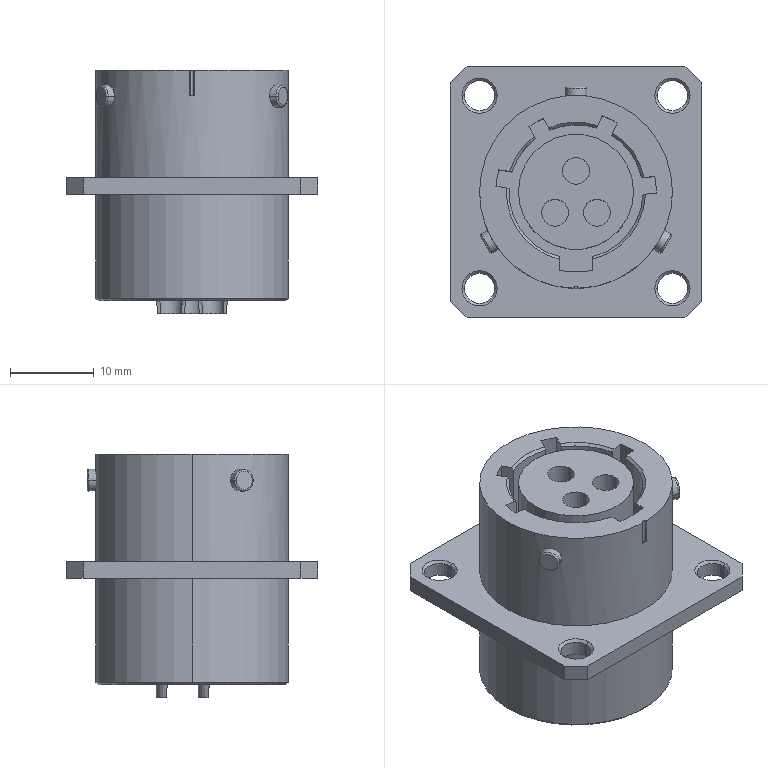Part | STEP file | Connector Y50DX5-1403Z30K | 1 solid | 128 faces | box 30 x 30 x 29.03 mm | volume 10352 mm3 | cylinder 59 | plane 44 | cone 17 | torus 8 | commonest cylinder face diameters 3.6 x14 16 x11 2.6 x6 3.2 x6 19.15 x5 23 x4